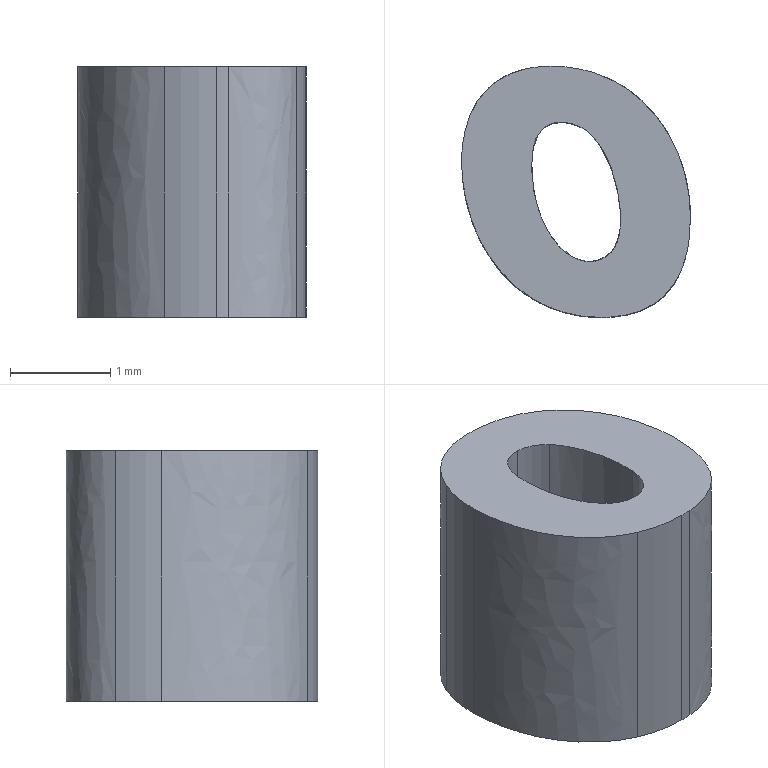Part | STEP file | lll_id1102_x_t | 1 solid | 17 faces | box 2.284 x 2.506 x 2.5 mm | volume 8.969 mm3 | other 9 | cylinder 6 | plane 2 | commonest cylinder face diameters 0.868 x1 2.315 x1 2.359 x1 2.639 x1 2.788 x1 2.85 x1
STEP:
#1=CARTESIAN_POINT('',(389.013,-124.465,2.35));
#2=VERTEX_POINT('',#1);
#3=CARTESIAN_POINT('',(389.328,-124.131,2.35));
#4=VERTEX_POINT('',#3);
#5=CARTESIAN_POINT('',(389.013,-124.465,2.35));
#6=CARTESIAN_POINT('',(389.141,-124.473,2.35));
#7=CARTESIAN_POINT('',(389.249,-124.404,2.35));
#8=CARTESIAN_POINT('',(389.303,-124.262,2.35));
#9=CARTESIAN_POINT('',(389.31,-124.24,2.35));
#10=CARTESIAN_POINT('',(389.322,-124.188,2.35));
#11=CARTESIAN_POINT('',(389.326,-124.16,2.35));
#12=CARTESIAN_POINT('',(389.328,-124.131,2.35));
#13=(BOUNDED_CURVE()B_SPLINE_CURVE(3,(#5,#6,#7,#8,#9,#10,#11,#12),.UNSPECIFIED.,.F.,.F.)B_SPLINE_CURVE_WITH_KNOTS((4,2,2,4),(0.,0.7103,0.842,1.),.UNSPECIFIED.)CURVE()GEOMETRIC_REPRESENTATION_ITEM()RATIONAL_B_SPLINE_CURVE((0.5541,0.482,0.482,0.5529,0.5529,0.5533,0.5533,0.5541))REPRESENTATION_ITEM(''));
#14=EDGE_CURVE('',#2,#4,#13,.T.);
#15=ORIENTED_EDGE('',*,*,#14,.T.);
#16=CARTESIAN_POINT('',(389.328,-124.131,-0.15));
#17=VERTEX_POINT('',#16);
#18=CARTESIAN_POINT('',(389.328,-124.131,-0.15));
#19=DIRECTION('',(0.,0.,1.));
#20=VECTOR('',#19,1.);
#21=LINE('',#18,#20);
#22=EDGE_CURVE('',#17,#4,#21,.T.);
#23=ORIENTED_EDGE('',*,*,#22,.F.);
#24=CARTESIAN_POINT('',(389.013,-124.465,-0.15));
#25=VERTEX_POINT('',#24);
#26=CARTESIAN_POINT('',(389.013,-124.465,-0.15));
#27=CARTESIAN_POINT('',(389.141,-124.473,-0.15));
#28=CARTESIAN_POINT('',(389.249,-124.404,-0.15));
#29=CARTESIAN_POINT('',(389.303,-124.262,-0.15));
#30=CARTESIAN_POINT('',(389.31,-124.24,-0.15));
#31=CARTESIAN_POINT('',(389.322,-124.188,-0.15));
#32=CARTESIAN_POINT('',(389.326,-124.16,-0.15));
#33=CARTESIAN_POINT('',(389.328,-124.131,-0.15));
#34=(BOUNDED_CURVE()B_SPLINE_CURVE(3,(#26,#27,#28,#29,#30,#31,#32,#33),.UNSPECIFIED.,.F.,.F.)B_SPLINE_CURVE_WITH_KNOTS((4,2,2,4),(0.,0.7103,0.842,1.),.UNSPECIFIED.)CURVE()GEOMETRIC_REPRESENTATION_ITEM()RATIONAL_B_SPLINE_CURVE((0.5541,0.482,0.482,0.5529,0.5529,0.5533,0.5533,0.5541))REPRESENTATION_ITEM(''));
#35=EDGE_CURVE('',#25,#17,#34,.T.);
#36=ORIENTED_EDGE('',*,*,#35,.F.);
#37=CARTESIAN_POINT('',(389.013,-124.465,-0.15));
#38=DIRECTION('',(0.,0.,1.));
#39=VECTOR('',#38,1.);
#40=LINE('',#37,#39);
#41=EDGE_CURVE('',#25,#2,#40,.T.);
#42=ORIENTED_EDGE('',*,*,#41,.T.);
#43=EDGE_LOOP('',(#15,#23,#36,#42));
#44=FACE_OUTER_BOUND('',#43,.T.);
#45=CARTESIAN_POINT('',(389.013,-124.465,-0.15));
#46=CARTESIAN_POINT('',(389.141,-124.473,-0.15));
#47=CARTESIAN_POINT('',(389.249,-124.404,-0.15));
#48=CARTESIAN_POINT('',(389.303,-124.262,-0.15));
#49=CARTESIAN_POINT('',(389.31,-124.24,-0.15));
#50=CARTESIAN_POINT('',(389.322,-124.188,-0.15));
#51=CARTESIAN_POINT('',(389.326,-124.16,-0.15));
#52=CARTESIAN_POINT('',(389.328,-124.131,-0.15));
#53=(BOUNDED_CURVE()B_SPLINE_CURVE(3,(#45,#46,#47,#48,#49,#50,#51,#52),.UNSPECIFIED.,.F.,.F.)B_SPLINE_CURVE_WITH_KNOTS((4,2,2,4),(0.,0.7103,0.842,1.),.UNSPECIFIED.)CURVE()GEOMETRIC_REPRESENTATION_ITEM()RATIONAL_B_SPLINE_CURVE((0.5541,0.482,0.482,0.5529,0.5529,0.5533,0.5533,0.5541))REPRESENTATION_ITEM(''));
#54=DIRECTION('',(0.,0.,1.));
#55=VECTOR('',#54,1.);
#56=SURFACE_OF_LINEAR_EXTRUSION('',#53,#55);
#57=ADVANCED_FACE('',(#44),#56,.F.);
#58=CARTESIAN_POINT('',(389.062,-123.223,2.35));
#59=VERTEX_POINT('',#58);
#60=CARTESIAN_POINT('',(389.328,-124.131,2.35));
#61=CARTESIAN_POINT('',(389.337,-124.008,2.35));
#62=CARTESIAN_POINT('',(389.329,-123.884,2.35));
#63=CARTESIAN_POINT('',(389.288,-123.679,2.35));
#64=CARTESIAN_POINT('',(389.265,-123.597,2.35));
#65=CARTESIAN_POINT('',(389.208,-123.446,2.35));
#66=CARTESIAN_POINT('',(389.173,-123.378,2.35));
#67=CARTESIAN_POINT('',(389.111,-123.282,2.35));
#68=CARTESIAN_POINT('',(389.088,-123.252,2.35));
#69=CARTESIAN_POINT('',(389.062,-123.223,2.35));
#70=(BOUNDED_CURVE()B_SPLINE_CURVE(3,(#60,#61,#62,#63,#64,#65,#66,#67,#68,#69),.UNSPECIFIED.,.F.,.F.)B_SPLINE_CURVE_WITH_KNOTS((4,2,2,2,4),(0.,0.3838,0.6481,0.8827,1.),.UNSPECIFIED.)CURVE()GEOMETRIC_REPRESENTATION_ITEM()RATIONAL_B_SPLINE_CURVE((0.5541,0.5507,0.5507,0.5528,0.5528,0.5521,0.5521,0.5529,0.5529,0.5541))REPRESENTATION_ITEM(''));
#71=EDGE_CURVE('',#4,#59,#70,.T.);
#72=ORIENTED_EDGE('',*,*,#71,.T.);
#73=CARTESIAN_POINT('',(389.062,-123.223,-0.15));
#74=VERTEX_POINT('',#73);
#75=CARTESIAN_POINT('',(389.062,-123.223,-0.15));
#76=DIRECTION('',(0.,0.,1.));
#77=VECTOR('',#76,1.);
#78=LINE('',#75,#77);
#79=EDGE_CURVE('',#74,#59,#78,.T.);
#80=ORIENTED_EDGE('',*,*,#79,.F.);
#81=CARTESIAN_POINT('',(389.328,-124.131,-0.15));
#82=CARTESIAN_POINT('',(389.337,-124.008,-0.15));
#83=CARTESIAN_POINT('',(389.329,-123.884,-0.15));
#84=CARTESIAN_POINT('',(389.288,-123.679,-0.15));
#85=CARTESIAN_POINT('',(389.265,-123.597,-0.15));
#86=CARTESIAN_POINT('',(389.208,-123.446,-0.15));
#87=CARTESIAN_POINT('',(389.173,-123.378,-0.15));
#88=CARTESIAN_POINT('',(389.111,-123.282,-0.15));
#89=CARTESIAN_POINT('',(389.088,-123.252,-0.15));
#90=CARTESIAN_POINT('',(389.062,-123.223,-0.15));
#91=(BOUNDED_CURVE()B_SPLINE_CURVE(3,(#81,#82,#83,#84,#85,#86,#87,#88,#89,#90),.UNSPECIFIED.,.F.,.F.)B_SPLINE_CURVE_WITH_KNOTS((4,2,2,2,4),(0.,0.3838,0.6481,0.8827,1.),.UNSPECIFIED.)CURVE()GEOMETRIC_REPRESENTATION_ITEM()RATIONAL_B_SPLINE_CURVE((0.5541,0.5507,0.5507,0.5528,0.5528,0.5521,0.5521,0.5529,0.5529,0.5541))REPRESENTATION_ITEM(''));
#92=EDGE_CURVE('',#17,#74,#91,.T.);
#93=ORIENTED_EDGE('',*,*,#92,.F.);
#94=ORIENTED_EDGE('',*,*,#22,.T.);
#95=EDGE_LOOP('',(#72,#80,#93,#94));
#96=FACE_OUTER_BOUND('',#95,.T.);
#97=CARTESIAN_POINT('',(389.328,-124.131,-0.15));
#98=CARTESIAN_POINT('',(389.337,-124.008,-0.15));
#99=CARTESIAN_POINT('',(389.329,-123.884,-0.15));
#100=CARTESIAN_POINT('',(389.288,-123.679,-0.15));
#101=CARTESIAN_POINT('',(389.265,-123.597,-0.15));
#102=CARTESIAN_POINT('',(389.208,-123.446,-0.15));
#103=CARTESIAN_POINT('',(389.173,-123.378,-0.15));
#104=CARTESIAN_POINT('',(389.111,-123.282,-0.15));
#105=CARTESIAN_POINT('',(389.088,-123.252,-0.15));
#106=CARTESIAN_POINT('',(389.062,-123.223,-0.15));
#107=(BOUNDED_CURVE()B_SPLINE_CURVE(3,(#97,#98,#99,#100,#101,#102,#103,#104,#105,#106),.UNSPECIFIED.,.F.,.F.)B_SPLINE_CURVE_WITH_KNOTS((4,2,2,2,4),(0.,0.3838,0.6481,0.8827,1.),.UNSPECIFIED.)CURVE()GEOMETRIC_REPRESENTATION_ITEM()RATIONAL_B_SPLINE_CURVE((0.5541,0.5507,0.5507,0.5528,0.5528,0.5521,0.5521,0.5529,0.5529,0.5541))REPRESENTATION_ITEM(''));
#108=DIRECTION('',(0.,0.,1.));
#109=VECTOR('',#108,1.);
#110=SURFACE_OF_LINEAR_EXTRUSION('',#107,#109);
#111=ADVANCED_FACE('',(#96),#110,.F.);
#112=CARTESIAN_POINT('',(388.763,-123.075,2.35));
#113=VERTEX_POINT('',#112);
#114=CARTESIAN_POINT('',(388.735,-123.509,2.35));
#115=DIRECTION('',(0.,0.,1.));
#116=DIRECTION('',(-1.,0.,0.));
#117=AXIS2_PLACEMENT_3D('',#114,#115,#116);
#118=CIRCLE('',#117,0.4341);
#119=EDGE_CURVE('',#59,#113,#118,.T.);
#120=ORIENTED_EDGE('',*,*,#119,.T.);
#121=CARTESIAN_POINT('',(388.763,-123.075,-0.15));
#122=VERTEX_POINT('',#121);
#123=CARTESIAN_POINT('',(388.763,-123.075,-0.15));
#124=DIRECTION('',(0.,0.,1.));
#125=VECTOR('',#124,1.);
#126=LINE('',#123,#125);
#127=EDGE_CURVE('',#122,#113,#126,.T.);
#128=ORIENTED_EDGE('',*,*,#127,.F.);
#129=CARTESIAN_POINT('',(388.735,-123.509,-0.15));
#130=DIRECTION('',(0.,0.,1.));
#131=DIRECTION('',(-1.,0.,0.));
#132=AXIS2_PLACEMENT_3D('',#129,#130,#131);
#133=CIRCLE('',#132,0.4341);
#134=EDGE_CURVE('',#74,#122,#133,.T.);
#135=ORIENTED_EDGE('',*,*,#134,.F.);
#136=ORIENTED_EDGE('',*,*,#79,.T.);
#137=EDGE_LOOP('',(#120,#128,#135,#136));
#138=FACE_OUTER_BOUND('',#137,.T.);
#139=CARTESIAN_POINT('',(388.735,-123.509,-0.15));
#140=DIRECTION('',(0.,0.,1.));
#141=DIRECTION('',(1.,0.,0.));
#142=AXIS2_PLACEMENT_3D('',#139,#140,#141);
#143=CYLINDRICAL_SURFACE('',#142,0.4341);
#144=ADVANCED_FACE('',(#138),#143,.F.);
#145=CARTESIAN_POINT('',(388.716,-124.311,2.35));
#146=VERTEX_POINT('',#145);
#147=CARTESIAN_POINT('',(388.763,-123.075,2.35));
#148=CARTESIAN_POINT('',(388.73,-123.073,2.35));
#149=CARTESIAN_POINT('',(388.696,-123.076,2.35));
#150=CARTESIAN_POINT('',(388.597,-123.1,2.35));
#151=CARTESIAN_POINT('',(388.542,-123.142,2.35));
#152=CARTESIAN_POINT('',(388.494,-123.227,2.35));
#153=CARTESIAN_POINT('',(388.483,-123.253,2.35));
#154=CARTESIAN_POINT('',(388.468,-123.304,2.35));
#155=CARTESIAN_POINT('',(388.463,-123.327,2.35));
#156=CARTESIAN_POINT('',(388.452,-123.388,2.35));
#157=CARTESIAN_POINT('',(388.448,-123.425,2.35));
#158=CARTESIAN_POINT('',(388.442,-123.606,2.35));
#159=CARTESIAN_POINT('',(388.459,-123.748,2.35));
#160=CARTESIAN_POINT('',(388.521,-123.987,2.35));
#161=CARTESIAN_POINT('',(388.562,-124.083,2.35));
#162=CARTESIAN_POINT('',(388.644,-124.222,2.35));
#163=CARTESIAN_POINT('',(388.678,-124.268,2.35));
#164=CARTESIAN_POINT('',(388.716,-124.311,2.35));
#165=(BOUNDED_CURVE()B_SPLINE_CURVE(3,(#147,#148,#149,#150,#151,#152,#153,#154,#155,#156,#157,#158,#159,#160,#161,#162,#163,#164),.UNSPECIFIED.,.F.,.F.)B_SPLINE_CURVE_WITH_KNOTS((4,2,2,2,2,2,2,2,4),(0.,0.07186,0.2116,0.2696,0.3174,0.394,0.6791,0.8867,1.),.UNSPECIFIED.)CURVE()GEOMETRIC_REPRESENTATION_ITEM()RATIONAL_B_SPLINE_CURVE((0.5028,0.4991,0.4991,0.4753,0.4753,0.5004,0.5004,0.5022,0.5022,0.502,0.502,0.4993,0.4993,0.4997,0.4997,0.5011,0.5011,0.5028))REPRESENTATION_ITEM(''));
#166=EDGE_CURVE('',#113,#146,#165,.T.);
#167=ORIENTED_EDGE('',*,*,#166,.T.);
#168=CARTESIAN_POINT('',(388.716,-124.311,-0.15));
#169=VERTEX_POINT('',#168);
#170=CARTESIAN_POINT('',(388.716,-124.311,-0.15));
#171=DIRECTION('',(0.,0.,1.));
#172=VECTOR('',#171,1.);
#173=LINE('',#170,#172);
#174=EDGE_CURVE('',#169,#146,#173,.T.);
#175=ORIENTED_EDGE('',*,*,#174,.F.);
#176=CARTESIAN_POINT('',(388.763,-123.075,-0.15));
#177=CARTESIAN_POINT('',(388.73,-123.073,-0.15));
#178=CARTESIAN_POINT('',(388.696,-123.076,-0.15));
#179=CARTESIAN_POINT('',(388.597,-123.1,-0.15));
#180=CARTESIAN_POINT('',(388.542,-123.142,-0.15));
#181=CARTESIAN_POINT('',(388.494,-123.227,-0.15));
#182=CARTESIAN_POINT('',(388.483,-123.253,-0.15));
#183=CARTESIAN_POINT('',(388.468,-123.304,-0.15));
#184=CARTESIAN_POINT('',(388.463,-123.327,-0.15));
#185=CARTESIAN_POINT('',(388.452,-123.388,-0.15));
#186=CARTESIAN_POINT('',(388.448,-123.425,-0.15));
#187=CARTESIAN_POINT('',(388.442,-123.606,-0.15));
#188=CARTESIAN_POINT('',(388.459,-123.748,-0.15));
#189=CARTESIAN_POINT('',(388.521,-123.987,-0.15));
#190=CARTESIAN_POINT('',(388.562,-124.083,-0.15));
#191=CARTESIAN_POINT('',(388.644,-124.222,-0.15));
#192=CARTESIAN_POINT('',(388.678,-124.268,-0.15));
#193=CARTESIAN_POINT('',(388.716,-124.311,-0.15));
#194=(BOUNDED_CURVE()B_SPLINE_CURVE(3,(#176,#177,#178,#179,#180,#181,#182,#183,#184,#185,#186,#187,#188,#189,#190,#191,#192,#193),.UNSPECIFIED.,.F.,.F.)B_SPLINE_CURVE_WITH_KNOTS((4,2,2,2,2,2,2,2,4),(0.,0.07186,0.2116,0.2696,0.3174,0.394,0.6791,0.8867,1.),.UNSPECIFIED.)CURVE()GEOMETRIC_REPRESENTATION_ITEM()RATIONAL_B_SPLINE_CURVE((0.5028,0.4991,0.4991,0.4753,0.4753,0.5004,0.5004,0.5022,0.5022,0.502,0.502,0.4993,0.4993,0.4997,0.4997,0.5011,0.5011,0.5028))REPRESENTATION_ITEM(''));
#195=EDGE_CURVE('',#122,#169,#194,.T.);
#196=ORIENTED_EDGE('',*,*,#195,.F.);
#197=ORIENTED_EDGE('',*,*,#127,.T.);
#198=EDGE_LOOP('',(#167,#175,#196,#197));
#199=FACE_OUTER_BOUND('',#198,.T.);
#200=CARTESIAN_POINT('',(388.763,-123.075,-0.15));
#201=CARTESIAN_POINT('',(388.73,-123.073,-0.15));
#202=CARTESIAN_POINT('',(388.696,-123.076,-0.15));
#203=CARTESIAN_POINT('',(388.597,-123.1,-0.15));
#204=CARTESIAN_POINT('',(388.542,-123.142,-0.15));
#205=CARTESIAN_POINT('',(388.494,-123.227,-0.15));
#206=CARTESIAN_POINT('',(388.483,-123.253,-0.15));
#207=CARTESIAN_POINT('',(388.468,-123.304,-0.15));
#208=CARTESIAN_POINT('',(388.463,-123.327,-0.15));
#209=CARTESIAN_POINT('',(388.452,-123.388,-0.15));
#210=CARTESIAN_POINT('',(388.448,-123.425,-0.15));
#211=CARTESIAN_POINT('',(388.442,-123.606,-0.15));
#212=CARTESIAN_POINT('',(388.459,-123.748,-0.15));
#213=CARTESIAN_POINT('',(388.521,-123.987,-0.15));
#214=CARTESIAN_POINT('',(388.562,-124.083,-0.15));
#215=CARTESIAN_POINT('',(388.644,-124.222,-0.15));
#216=CARTESIAN_POINT('',(388.678,-124.268,-0.15));
#217=CARTESIAN_POINT('',(388.716,-124.311,-0.15));
#218=(BOUNDED_CURVE()B_SPLINE_CURVE(3,(#200,#201,#202,#203,#204,#205,#206,#207,#208,#209,#210,#211,#212,#213,#214,#215,#216,#217),.UNSPECIFIED.,.F.,.F.)B_SPLINE_CURVE_WITH_KNOTS((4,2,2,2,2,2,2,2,4),(0.,0.07186,0.2116,0.2696,0.3174,0.394,0.6791,0.8867,1.),.UNSPECIFIED.)CURVE()GEOMETRIC_REPRESENTATION_ITEM()RATIONAL_B_SPLINE_CURVE((0.5028,0.4991,0.4991,0.4753,0.4753,0.5004,0.5004,0.5022,0.5022,0.502,0.502,0.4993,0.4993,0.4997,0.4997,0.5011,0.5011,0.5028))REPRESENTATION_ITEM(''));
#219=DIRECTION('',(0.,0.,1.));
#220=VECTOR('',#219,1.);
#221=SURFACE_OF_LINEAR_EXTRUSION('',#218,#220);
#222=ADVANCED_FACE('',(#199),#221,.F.);
#223=CARTESIAN_POINT('',(388.984,-124.463,2.35));
#224=VERTEX_POINT('',#223);
#225=CARTESIAN_POINT('',(388.716,-124.311,2.35));
#226=CARTESIAN_POINT('',(388.757,-124.358,2.35));
#227=CARTESIAN_POINT('',(388.806,-124.396,2.35));
#228=CARTESIAN_POINT('',(388.9,-124.446,2.35));
#229=CARTESIAN_POINT('',(388.941,-124.459,2.35));
#230=CARTESIAN_POINT('',(388.984,-124.463,2.35));
#231=(BOUNDED_CURVE()B_SPLINE_CURVE(3,(#225,#226,#227,#228,#229,#230),.UNSPECIFIED.,.F.,.F.)B_SPLINE_CURVE_WITH_KNOTS((4,2,4),(0.,0.5929,1.),.UNSPECIFIED.)CURVE()GEOMETRIC_REPRESENTATION_ITEM()RATIONAL_B_SPLINE_CURVE((0.5028,0.4974,0.4974,0.497,0.497,0.5028))REPRESENTATION_ITEM(''));
#232=EDGE_CURVE('',#146,#224,#231,.T.);
#233=ORIENTED_EDGE('',*,*,#232,.T.);
#234=CARTESIAN_POINT('',(388.984,-124.463,-0.15));
#235=VERTEX_POINT('',#234);
#236=CARTESIAN_POINT('',(388.984,-124.463,-0.15));
#237=DIRECTION('',(0.,0.,1.));
#238=VECTOR('',#237,1.);
#239=LINE('',#236,#238);
#240=EDGE_CURVE('',#235,#224,#239,.T.);
#241=ORIENTED_EDGE('',*,*,#240,.F.);
#242=CARTESIAN_POINT('',(388.716,-124.311,-0.15));
#243=CARTESIAN_POINT('',(388.757,-124.358,-0.15));
#244=CARTESIAN_POINT('',(388.806,-124.396,-0.15));
#245=CARTESIAN_POINT('',(388.9,-124.446,-0.15));
#246=CARTESIAN_POINT('',(388.941,-124.459,-0.15));
#247=CARTESIAN_POINT('',(388.984,-124.463,-0.15));
#248=(BOUNDED_CURVE()B_SPLINE_CURVE(3,(#242,#243,#244,#245,#246,#247),.UNSPECIFIED.,.F.,.F.)B_SPLINE_CURVE_WITH_KNOTS((4,2,4),(0.,0.5929,1.),.UNSPECIFIED.)CURVE()GEOMETRIC_REPRESENTATION_ITEM()RATIONAL_B_SPLINE_CURVE((0.5028,0.4974,0.4974,0.497,0.497,0.5028))REPRESENTATION_ITEM(''));
#249=EDGE_CURVE('',#169,#235,#248,.T.);
#250=ORIENTED_EDGE('',*,*,#249,.F.);
#251=ORIENTED_EDGE('',*,*,#174,.T.);
#252=EDGE_LOOP('',(#233,#241,#250,#251));
#253=FACE_OUTER_BOUND('',#252,.T.);
#254=CARTESIAN_POINT('',(388.716,-124.311,-0.15));
#255=CARTESIAN_POINT('',(388.757,-124.358,-0.15));
#256=CARTESIAN_POINT('',(388.806,-124.396,-0.15));
#257=CARTESIAN_POINT('',(388.9,-124.446,-0.15));
#258=CARTESIAN_POINT('',(388.941,-124.459,-0.15));
#259=CARTESIAN_POINT('',(388.984,-124.463,-0.15));
#260=(BOUNDED_CURVE()B_SPLINE_CURVE(3,(#254,#255,#256,#257,#258,#259),.UNSPECIFIED.,.F.,.F.)B_SPLINE_CURVE_WITH_KNOTS((4,2,4),(0.,0.5929,1.),.UNSPECIFIED.)CURVE()GEOMETRIC_REPRESENTATION_ITEM()RATIONAL_B_SPLINE_CURVE((0.5028,0.4974,0.4974,0.497,0.497,0.5028))REPRESENTATION_ITEM(''));
#261=DIRECTION('',(0.,0.,1.));
#262=VECTOR('',#261,1.);
#263=SURFACE_OF_LINEAR_EXTRUSION('',#260,#262);
#264=ADVANCED_FACE('',(#253),#263,.F.);
#265=CARTESIAN_POINT('',(388.65,-122.517,2.35));
#266=VERTEX_POINT('',#265);
#267=CARTESIAN_POINT('',(389.061,-122.579,2.35));
#268=VERTEX_POINT('',#267);
#269=CARTESIAN_POINT('',(388.645,-123.942,2.35));
#270=DIRECTION('',(0.,0.,-1.));
#271=DIRECTION('',(0.,-1.,0.));
#272=AXIS2_PLACEMENT_3D('',#269,#270,#271);
#273=CIRCLE('',#272,1.425);
#274=EDGE_CURVE('',#266,#268,#273,.T.);
#275=ORIENTED_EDGE('',*,*,#274,.T.);
#276=CARTESIAN_POINT('',(389.061,-122.579,-0.15));
#277=VERTEX_POINT('',#276);
#278=CARTESIAN_POINT('',(389.061,-122.579,-0.15));
#279=DIRECTION('',(0.,0.,1.));
#280=VECTOR('',#279,1.);
#281=LINE('',#278,#280);
#282=EDGE_CURVE('',#277,#268,#281,.T.);
#283=ORIENTED_EDGE('',*,*,#282,.F.);
#284=CARTESIAN_POINT('',(388.65,-122.517,-0.15));
#285=VERTEX_POINT('',#284);
#286=CARTESIAN_POINT('',(388.645,-123.942,-0.15));
#287=DIRECTION('',(0.,0.,-1.));
#288=DIRECTION('',(1.,0.,0.));
#289=AXIS2_PLACEMENT_3D('',#286,#287,#288);
#290=CIRCLE('',#289,1.425);
#291=EDGE_CURVE('',#285,#277,#290,.T.);
#292=ORIENTED_EDGE('',*,*,#291,.F.);
#293=CARTESIAN_POINT('',(388.65,-122.517,-0.15));
#294=DIRECTION('',(0.,0.,1.));
#295=VECTOR('',#294,1.);
#296=LINE('',#293,#295);
#297=EDGE_CURVE('',#285,#266,#296,.T.);
#298=ORIENTED_EDGE('',*,*,#297,.T.);
#299=EDGE_LOOP('',(#275,#283,#292,#298));
#300=FACE_OUTER_BOUND('',#299,.T.);
#301=CARTESIAN_POINT('',(388.645,-123.942,-0.15));
#302=DIRECTION('',(0.,0.,1.));
#303=DIRECTION('',(1.,0.,0.));
#304=AXIS2_PLACEMENT_3D('',#301,#302,#303);
#305=CYLINDRICAL_SURFACE('',#304,1.425);
#306=ADVANCED_FACE('',(#300),#305,.T.);
#307=CARTESIAN_POINT('',(390.017,-124.245,2.35));
#308=VERTEX_POINT('',#307);
#309=CARTESIAN_POINT('',(389.061,-122.579,2.35));
#310=CARTESIAN_POINT('',(389.291,-122.652,2.35));
#311=CARTESIAN_POINT('',(389.492,-122.785,2.35));
#312=CARTESIAN_POINT('',(389.805,-123.151,2.35));
#313=CARTESIAN_POINT('',(389.917,-123.363,2.35));
#314=CARTESIAN_POINT('',(390.03,-123.808,2.35));
#315=CARTESIAN_POINT('',(390.044,-124.028,2.35));
#316=CARTESIAN_POINT('',(390.017,-124.245,2.35));
#317=(BOUNDED_CURVE()B_SPLINE_CURVE(3,(#309,#310,#311,#312,#313,#314,#315,#316),.UNSPECIFIED.,.F.,.F.)B_SPLINE_CURVE_WITH_KNOTS((4,2,2,4),(0.,0.3492,0.691,1.),.UNSPECIFIED.)CURVE()GEOMETRIC_REPRESENTATION_ITEM()RATIONAL_B_SPLINE_CURVE((0.5027,0.4899,0.4899,0.4938,0.4938,0.4968,0.4968,0.5027))REPRESENTATION_ITEM(''));
#318=EDGE_CURVE('',#268,#308,#317,.T.);
#319=ORIENTED_EDGE('',*,*,#318,.T.);
#320=CARTESIAN_POINT('',(390.017,-124.245,-0.15));
#321=VERTEX_POINT('',#320);
#322=CARTESIAN_POINT('',(390.017,-124.245,-0.15));
#323=DIRECTION('',(0.,0.,1.));
#324=VECTOR('',#323,1.);
#325=LINE('',#322,#324);
#326=EDGE_CURVE('',#321,#308,#325,.T.);
#327=ORIENTED_EDGE('',*,*,#326,.F.);
#328=CARTESIAN_POINT('',(389.061,-122.579,-0.15));
#329=CARTESIAN_POINT('',(389.291,-122.652,-0.15));
#330=CARTESIAN_POINT('',(389.492,-122.785,-0.15));
#331=CARTESIAN_POINT('',(389.805,-123.151,-0.15));
#332=CARTESIAN_POINT('',(389.917,-123.363,-0.15));
#333=CARTESIAN_POINT('',(390.03,-123.808,-0.15));
#334=CARTESIAN_POINT('',(390.044,-124.028,-0.15));
#335=CARTESIAN_POINT('',(390.017,-124.245,-0.15));
#336=(BOUNDED_CURVE()B_SPLINE_CURVE(3,(#328,#329,#330,#331,#332,#333,#334,#335),.UNSPECIFIED.,.F.,.F.)B_SPLINE_CURVE_WITH_KNOTS((4,2,2,4),(0.,0.3492,0.691,1.),.UNSPECIFIED.)CURVE()GEOMETRIC_REPRESENTATION_ITEM()RATIONAL_B_SPLINE_CURVE((0.5027,0.4899,0.4899,0.4938,0.4938,0.4968,0.4968,0.5027))REPRESENTATION_ITEM(''));
#337=EDGE_CURVE('',#277,#321,#336,.T.);
#338=ORIENTED_EDGE('',*,*,#337,.F.);
#339=ORIENTED_EDGE('',*,*,#282,.T.);
#340=EDGE_LOOP('',(#319,#327,#338,#339));
#341=FACE_OUTER_BOUND('',#340,.T.);
#342=CARTESIAN_POINT('',(389.061,-122.579,-0.15));
#343=CARTESIAN_POINT('',(389.291,-122.652,-0.15));
#344=CARTESIAN_POINT('',(389.492,-122.785,-0.15));
#345=CARTESIAN_POINT('',(389.805,-123.151,-0.15));
#346=CARTESIAN_POINT('',(389.917,-123.363,-0.15));
#347=CARTESIAN_POINT('',(390.03,-123.808,-0.15));
#348=CARTESIAN_POINT('',(390.044,-124.028,-0.15));
#349=CARTESIAN_POINT('',(390.017,-124.245,-0.15));
#350=(BOUNDED_CURVE()B_SPLINE_CURVE(3,(#342,#343,#344,#345,#346,#347,#348,#349),.UNSPECIFIED.,.F.,.F.)B_SPLINE_CURVE_WITH_KNOTS((4,2,2,4),(0.,0.3492,0.691,1.),.UNSPECIFIED.)CURVE()GEOMETRIC_REPRESENTATION_ITEM()RATIONAL_B_SPLINE_CURVE((0.5027,0.4899,0.4899,0.4938,0.4938,0.4968,0.4968,0.5027))REPRESENTATION_ITEM(''));
#351=DIRECTION('',(0.,0.,1.));
#352=VECTOR('',#351,1.);
#353=SURFACE_OF_LINEAR_EXTRUSION('',#350,#352);
#354=ADVANCED_FACE('',(#341),#353,.F.);
#355=CARTESIAN_POINT('',(389.934,-124.562,2.35));
#356=VERTEX_POINT('',#355);
#357=CARTESIAN_POINT('',(388.845,-124.109,2.35));
#358=DIRECTION('',(0.,0.,-1.));
#359=DIRECTION('',(1.,0.,0.));
#360=AXIS2_PLACEMENT_3D('',#357,#358,#359);
#361=CIRCLE('',#360,1.179);
#362=EDGE_CURVE('',#308,#356,#361,.T.);
#363=ORIENTED_EDGE('',*,*,#362,.T.);
#364=CARTESIAN_POINT('',(389.934,-124.562,-0.15));
#365=VERTEX_POINT('',#364);
#366=CARTESIAN_POINT('',(389.934,-124.562,-0.15));
#367=DIRECTION('',(0.,0.,1.));
#368=VECTOR('',#367,1.);
#369=LINE('',#366,#368);
#370=EDGE_CURVE('',#365,#356,#369,.T.);
#371=ORIENTED_EDGE('',*,*,#370,.F.);
#372=CARTESIAN_POINT('',(388.845,-124.109,-0.15));
#373=DIRECTION('',(0.,0.,-1.));
#374=DIRECTION('',(1.,0.,0.));
#375=AXIS2_PLACEMENT_3D('',#372,#373,#374);
#376=CIRCLE('',#375,1.179);
#377=EDGE_CURVE('',#321,#365,#376,.T.);
#378=ORIENTED_EDGE('',*,*,#377,.F.);
#379=ORIENTED_EDGE('',*,*,#326,.T.);
#380=EDGE_LOOP('',(#363,#371,#378,#379));
#381=FACE_OUTER_BOUND('',#380,.T.);
#382=CARTESIAN_POINT('',(388.845,-124.109,-0.15));
#383=DIRECTION('',(0.,0.,1.));
#384=DIRECTION('',(1.,0.,0.));
#385=AXIS2_PLACEMENT_3D('',#382,#383,#384);
#386=CYLINDRICAL_SURFACE('',#385,1.179);
#387=ADVANCED_FACE('',(#381),#386,.T.);
#388=CARTESIAN_POINT('',(389.253,-125.018,2.35));
#389=VERTEX_POINT('',#388);
#390=CARTESIAN_POINT('',(389.934,-124.562,2.35));
#391=CARTESIAN_POINT('',(389.857,-124.753,2.35));
#392=CARTESIAN_POINT('',(389.709,-124.895,2.35));
#393=CARTESIAN_POINT('',(389.43,-124.993,2.35));
#394=CARTESIAN_POINT('',(389.343,-125.011,2.35));
#395=CARTESIAN_POINT('',(389.253,-125.018,2.35));
#396=(BOUNDED_CURVE()B_SPLINE_CURVE(3,(#390,#391,#392,#393,#394,#395),.UNSPECIFIED.,.F.,.F.)B_SPLINE_CURVE_WITH_KNOTS((4,2,4),(0.,0.698,1.),.UNSPECIFIED.)CURVE()GEOMETRIC_REPRESENTATION_ITEM()RATIONAL_B_SPLINE_CURVE((0.5027,0.4728,0.4728,0.4997,0.4997,0.5027))REPRESENTATION_ITEM(''));
#397=EDGE_CURVE('',#356,#389,#396,.T.);
#398=ORIENTED_EDGE('',*,*,#397,.T.);
#399=CARTESIAN_POINT('',(389.253,-125.018,-0.15));
#400=VERTEX_POINT('',#399);
#401=CARTESIAN_POINT('',(389.253,-125.018,-0.15));
#402=DIRECTION('',(0.,0.,1.));
#403=VECTOR('',#402,1.);
#404=LINE('',#401,#403);
#405=EDGE_CURVE('',#400,#389,#404,.T.);
#406=ORIENTED_EDGE('',*,*,#405,.F.);
#407=CARTESIAN_POINT('',(389.934,-124.562,-0.15));
#408=CARTESIAN_POINT('',(389.857,-124.753,-0.15));
#409=CARTESIAN_POINT('',(389.709,-124.895,-0.15));
#410=CARTESIAN_POINT('',(389.43,-124.993,-0.15));
#411=CARTESIAN_POINT('',(389.343,-125.011,-0.15));
#412=CARTESIAN_POINT('',(389.253,-125.018,-0.15));
#413=(BOUNDED_CURVE()B_SPLINE_CURVE(3,(#407,#408,#409,#410,#411,#412),.UNSPECIFIED.,.F.,.F.)B_SPLINE_CURVE_WITH_KNOTS((4,2,4),(0.,0.698,1.),.UNSPECIFIED.)CURVE()GEOMETRIC_REPRESENTATION_ITEM()RATIONAL_B_SPLINE_CURVE((0.5027,0.4728,0.4728,0.4997,0.4997,0.5027))REPRESENTATION_ITEM(''));
#414=EDGE_CURVE('',#365,#400,#413,.T.);
#415=ORIENTED_EDGE('',*,*,#414,.F.);
#416=ORIENTED_EDGE('',*,*,#370,.T.);
#417=EDGE_LOOP('',(#398,#406,#415,#416));
#418=FACE_OUTER_BOUND('',#417,.T.);
#419=CARTESIAN_POINT('',(389.934,-124.562,-0.15));
#420=CARTESIAN_POINT('',(389.857,-124.753,-0.15));
#421=CARTESIAN_POINT('',(389.709,-124.895,-0.15));
#422=CARTESIAN_POINT('',(389.43,-124.993,-0.15));
#423=CARTESIAN_POINT('',(389.343,-125.011,-0.15));
#424=CARTESIAN_POINT('',(389.253,-125.018,-0.15));
#425=(BOUNDED_CURVE()B_SPLINE_CURVE(3,(#419,#420,#421,#422,#423,#424),.UNSPECIFIED.,.F.,.F.)B_SPLINE_CURVE_WITH_KNOTS((4,2,4),(0.,0.698,1.),.UNSPECIFIED.)CURVE()GEOMETRIC_REPRESENTATION_ITEM()RATIONAL_B_SPLINE_CURVE((0.5027,0.4728,0.4728,0.4997,0.4997,0.5027))REPRESENTATION_ITEM(''));
#426=DIRECTION('',(0.,0.,1.));
#427=VECTOR('',#426,1.);
#428=SURFACE_OF_LINEAR_EXTRUSION('',#425,#427);
#429=ADVANCED_FACE('',(#418),#428,.F.);
#430=CARTESIAN_POINT('',(389.135,-125.023,2.35));
#431=VERTEX_POINT('',#430);
#432=CARTESIAN_POINT('',(389.139,-123.629,2.35));
#433=DIRECTION('',(0.,0.,-1.));
#434=DIRECTION('',(0.,-1.,0.));
#435=AXIS2_PLACEMENT_3D('',#432,#433,#434);
#436=CIRCLE('',#435,1.394);
#437=EDGE_CURVE('',#389,#431,#436,.T.);
#438=ORIENTED_EDGE('',*,*,#437,.T.);
#439=CARTESIAN_POINT('',(389.135,-125.023,-0.15));
#440=VERTEX_POINT('',#439);
#441=CARTESIAN_POINT('',(389.135,-125.023,-0.15));
#442=DIRECTION('',(0.,0.,1.));
#443=VECTOR('',#442,1.);
#444=LINE('',#441,#443);
#445=EDGE_CURVE('',#440,#431,#444,.T.);
#446=ORIENTED_EDGE('',*,*,#445,.F.);
#447=CARTESIAN_POINT('',(389.139,-123.629,-0.15));
#448=DIRECTION('',(0.,0.,-1.));
#449=DIRECTION('',(0.,-1.,0.));
#450=AXIS2_PLACEMENT_3D('',#447,#448,#449);
#451=CIRCLE('',#450,1.394);
#452=EDGE_CURVE('',#400,#440,#451,.T.);
#453=ORIENTED_EDGE('',*,*,#452,.F.);
#454=ORIENTED_EDGE('',*,*,#405,.T.);
#455=EDGE_LOOP('',(#438,#446,#453,#454));
#456=FACE_OUTER_BOUND('',#455,.T.);
#457=CARTESIAN_POINT('',(389.139,-123.629,-0.15));
#458=DIRECTION('',(0.,0.,1.));
#459=DIRECTION('',(1.,0.,0.));
#460=AXIS2_PLACEMENT_3D('',#457,#458,#459);
#461=CYLINDRICAL_SURFACE('',#460,1.394);
#462=ADVANCED_FACE('',(#456),#461,.T.);
#463=CARTESIAN_POINT('',(388.612,-124.918,2.35));
#464=VERTEX_POINT('',#463);
#465=CARTESIAN_POINT('',(389.127,-123.703,2.35));
#466=DIRECTION('',(0.,0.,-1.));
#467=DIRECTION('',(1.,0.,0.));
#468=AXIS2_PLACEMENT_3D('',#465,#466,#467);
#469=CIRCLE('',#468,1.319);
#470=EDGE_CURVE('',#431,#464,#469,.T.);
#471=ORIENTED_EDGE('',*,*,#470,.T.);
#472=CARTESIAN_POINT('',(388.612,-124.918,-0.15));
#473=VERTEX_POINT('',#472);
#474=CARTESIAN_POINT('',(388.612,-124.918,-0.15));
#475=DIRECTION('',(0.,0.,1.));
#476=VECTOR('',#475,1.);
#477=LINE('',#474,#476);
#478=EDGE_CURVE('',#473,#464,#477,.T.);
#479=ORIENTED_EDGE('',*,*,#478,.F.);
#480=CARTESIAN_POINT('',(389.127,-123.703,-0.15));
#481=DIRECTION('',(0.,0.,-1.));
#482=DIRECTION('',(1.,0.,0.));
#483=AXIS2_PLACEMENT_3D('',#480,#481,#482);
#484=CIRCLE('',#483,1.319);
#485=EDGE_CURVE('',#440,#473,#484,.T.);
#486=ORIENTED_EDGE('',*,*,#485,.F.);
#487=ORIENTED_EDGE('',*,*,#445,.T.);
#488=EDGE_LOOP('',(#471,#479,#486,#487));
#489=FACE_OUTER_BOUND('',#488,.T.);
#490=CARTESIAN_POINT('',(389.127,-123.703,-0.15));
#491=DIRECTION('',(0.,0.,1.));
#492=DIRECTION('',(1.,0.,0.));
#493=AXIS2_PLACEMENT_3D('',#490,#491,#492);
#494=CYLINDRICAL_SURFACE('',#493,1.319);
#495=ADVANCED_FACE('',(#489),#494,.T.);
#496=CARTESIAN_POINT('',(387.746,-123.469,2.35));
#497=VERTEX_POINT('',#496);
#498=CARTESIAN_POINT('',(388.612,-124.918,2.35));
#499=CARTESIAN_POINT('',(388.41,-124.83,2.35));
#500=CARTESIAN_POINT('',(388.236,-124.695,2.35));
#501=CARTESIAN_POINT('',(387.99,-124.38,2.35));
#502=CARTESIAN_POINT('',(387.905,-124.222,2.35));
#503=CARTESIAN_POINT('',(387.783,-123.864,2.35));
#504=CARTESIAN_POINT('',(387.749,-123.668,2.35));
#505=CARTESIAN_POINT('',(387.746,-123.469,2.35));
#506=(BOUNDED_CURVE()B_SPLINE_CURVE(3,(#498,#499,#500,#501,#502,#503,#504,#505),.UNSPECIFIED.,.F.,.F.)B_SPLINE_CURVE_WITH_KNOTS((4,2,2,4),(0.,0.3712,0.6704,1.),.UNSPECIFIED.)CURVE()GEOMETRIC_REPRESENTATION_ITEM()RATIONAL_B_SPLINE_CURVE((0.5052,0.4949,0.4949,0.5005,0.5005,0.5009,0.5009,0.5052))REPRESENTATION_ITEM(''));
#507=EDGE_CURVE('',#464,#497,#506,.T.);
#508=ORIENTED_EDGE('',*,*,#507,.T.);
#509=CARTESIAN_POINT('',(387.746,-123.469,-0.15));
#510=VERTEX_POINT('',#509);
#511=CARTESIAN_POINT('',(387.746,-123.469,-0.15));
#512=DIRECTION('',(0.,0.,1.));
#513=VECTOR('',#512,1.);
#514=LINE('',#511,#513);
#515=EDGE_CURVE('',#510,#497,#514,.T.);
#516=ORIENTED_EDGE('',*,*,#515,.F.);
#517=CARTESIAN_POINT('',(388.612,-124.918,-0.15));
#518=CARTESIAN_POINT('',(388.41,-124.83,-0.15));
#519=CARTESIAN_POINT('',(388.236,-124.695,-0.15));
#520=CARTESIAN_POINT('',(387.99,-124.38,-0.15));
#521=CARTESIAN_POINT('',(387.905,-124.222,-0.15));
#522=CARTESIAN_POINT('',(387.783,-123.864,-0.15));
#523=CARTESIAN_POINT('',(387.749,-123.668,-0.15));
#524=CARTESIAN_POINT('',(387.746,-123.469,-0.15));
#525=(BOUNDED_CURVE()B_SPLINE_CURVE(3,(#517,#518,#519,#520,#521,#522,#523,#524),.UNSPECIFIED.,.F.,.F.)B_SPLINE_CURVE_WITH_KNOTS((4,2,2,4),(0.,0.3712,0.6704,1.),.UNSPECIFIED.)CURVE()GEOMETRIC_REPRESENTATION_ITEM()RATIONAL_B_SPLINE_CURVE((0.5052,0.4949,0.4949,0.5005,0.5005,0.5009,0.5009,0.5052))REPRESENTATION_ITEM(''));
#526=EDGE_CURVE('',#473,#510,#525,.T.);
#527=ORIENTED_EDGE('',*,*,#526,.F.);
#528=ORIENTED_EDGE('',*,*,#478,.T.);
#529=EDGE_LOOP('',(#508,#516,#527,#528));
#530=FACE_OUTER_BOUND('',#529,.T.);
#531=CARTESIAN_POINT('',(388.612,-124.918,-0.15));
#532=CARTESIAN_POINT('',(388.41,-124.83,-0.15));
#533=CARTESIAN_POINT('',(388.236,-124.695,-0.15));
#534=CARTESIAN_POINT('',(387.99,-124.38,-0.15));
#535=CARTESIAN_POINT('',(387.905,-124.222,-0.15));
#536=CARTESIAN_POINT('',(387.783,-123.864,-0.15));
#537=CARTESIAN_POINT('',(387.749,-123.668,-0.15));
#538=CARTESIAN_POINT('',(387.746,-123.469,-0.15));
#539=(BOUNDED_CURVE()B_SPLINE_CURVE(3,(#531,#532,#533,#534,#535,#536,#537,#538),.UNSPECIFIED.,.F.,.F.)B_SPLINE_CURVE_WITH_KNOTS((4,2,2,4),(0.,0.3712,0.6704,1.),.UNSPECIFIED.)CURVE()GEOMETRIC_REPRESENTATION_ITEM()RATIONAL_B_SPLINE_CURVE((0.5052,0.4949,0.4949,0.5005,0.5005,0.5009,0.5009,0.5052))REPRESENTATION_ITEM(''));
#540=DIRECTION('',(0.,0.,1.));
#541=VECTOR('',#540,1.);
#542=SURFACE_OF_LINEAR_EXTRUSION('',#539,#541);
#543=ADVANCED_FACE('',(#530),#542,.F.);
#544=CARTESIAN_POINT('',(387.833,-123.003,2.35));
#545=VERTEX_POINT('',#544);
#546=CARTESIAN_POINT('',(388.904,-123.444,2.35));
#547=DIRECTION('',(0.,0.,-1.));
#548=DIRECTION('',(1.,0.,0.));
#549=AXIS2_PLACEMENT_3D('',#546,#547,#548);
#550=CIRCLE('',#549,1.157);
#551=EDGE_CURVE('',#497,#545,#550,.T.);
#552=ORIENTED_EDGE('',*,*,#551,.T.);
#553=CARTESIAN_POINT('',(387.833,-123.003,-0.15));
#554=VERTEX_POINT('',#553);
#555=CARTESIAN_POINT('',(387.833,-123.003,-0.15));
#556=DIRECTION('',(0.,0.,1.));
#557=VECTOR('',#556,1.);
#558=LINE('',#555,#557);
#559=EDGE_CURVE('',#554,#545,#558,.T.);
#560=ORIENTED_EDGE('',*,*,#559,.F.);
#561=CARTESIAN_POINT('',(388.904,-123.444,-0.15));
#562=DIRECTION('',(0.,0.,-1.));
#563=DIRECTION('',(1.,0.,0.));
#564=AXIS2_PLACEMENT_3D('',#561,#562,#563);
#565=CIRCLE('',#564,1.157);
#566=EDGE_CURVE('',#510,#554,#565,.T.);
#567=ORIENTED_EDGE('',*,*,#566,.F.);
#568=ORIENTED_EDGE('',*,*,#515,.T.);
#569=EDGE_LOOP('',(#552,#560,#567,#568));
#570=FACE_OUTER_BOUND('',#569,.T.);
#571=CARTESIAN_POINT('',(388.904,-123.444,-0.15));
#572=DIRECTION('',(0.,0.,1.));
#573=DIRECTION('',(1.,0.,0.));
#574=AXIS2_PLACEMENT_3D('',#571,#572,#573);
#575=CYLINDRICAL_SURFACE('',#574,1.157);
#576=ADVANCED_FACE('',(#570),#575,.T.);
#577=CARTESIAN_POINT('',(387.833,-123.003,2.35));
#578=CARTESIAN_POINT('',(387.921,-122.783,2.35));
#579=CARTESIAN_POINT('',(388.098,-122.624,2.35));
#580=CARTESIAN_POINT('',(388.393,-122.54,2.35));
#581=CARTESIAN_POINT('',(388.462,-122.527,2.35));
#582=CARTESIAN_POINT('',(388.571,-122.518,2.35));
#583=CARTESIAN_POINT('',(388.61,-122.517,2.35));
#584=CARTESIAN_POINT('',(388.65,-122.517,2.35));
#585=(BOUNDED_CURVE()B_SPLINE_CURVE(3,(#577,#578,#579,#580,#581,#582,#583,#584),.UNSPECIFIED.,.F.,.F.)B_SPLINE_CURVE_WITH_KNOTS((4,2,2,4),(0.,0.6854,0.8859,1.),.UNSPECIFIED.)CURVE()GEOMETRIC_REPRESENTATION_ITEM()RATIONAL_B_SPLINE_CURVE((0.5052,0.4708,0.4708,0.5034,0.5034,0.5049,0.5049,0.5052))REPRESENTATION_ITEM(''));
#586=EDGE_CURVE('',#545,#266,#585,.T.);
#587=ORIENTED_EDGE('',*,*,#586,.T.);
#588=ORIENTED_EDGE('',*,*,#297,.F.);
#589=CARTESIAN_POINT('',(387.833,-123.003,-0.15));
#590=CARTESIAN_POINT('',(387.921,-122.783,-0.15));
#591=CARTESIAN_POINT('',(388.098,-122.624,-0.15));
#592=CARTESIAN_POINT('',(388.393,-122.54,-0.15));
#593=CARTESIAN_POINT('',(388.462,-122.527,-0.15));
#594=CARTESIAN_POINT('',(388.571,-122.518,-0.15));
#595=CARTESIAN_POINT('',(388.61,-122.517,-0.15));
#596=CARTESIAN_POINT('',(388.65,-122.517,-0.15));
#597=(BOUNDED_CURVE()B_SPLINE_CURVE(3,(#589,#590,#591,#592,#593,#594,#595,#596),.UNSPECIFIED.,.F.,.F.)B_SPLINE_CURVE_WITH_KNOTS((4,2,2,4),(0.,0.6854,0.8859,1.),.UNSPECIFIED.)CURVE()GEOMETRIC_REPRESENTATION_ITEM()RATIONAL_B_SPLINE_CURVE((0.5052,0.4708,0.4708,0.5034,0.5034,0.5049,0.5049,0.5052))REPRESENTATION_ITEM(''));
#598=EDGE_CURVE('',#554,#285,#597,.T.);
#599=ORIENTED_EDGE('',*,*,#598,.F.);
#600=ORIENTED_EDGE('',*,*,#559,.T.);
#601=EDGE_LOOP('',(#587,#588,#599,#600));
#602=FACE_OUTER_BOUND('',#601,.T.);
#603=CARTESIAN_POINT('',(387.833,-123.003,-0.15));
#604=CARTESIAN_POINT('',(387.921,-122.783,-0.15));
#605=CARTESIAN_POINT('',(388.098,-122.624,-0.15));
#606=CARTESIAN_POINT('',(388.393,-122.54,-0.15));
#607=CARTESIAN_POINT('',(388.462,-122.527,-0.15));
#608=CARTESIAN_POINT('',(388.571,-122.518,-0.15));
#609=CARTESIAN_POINT('',(388.61,-122.517,-0.15));
#610=CARTESIAN_POINT('',(388.65,-122.517,-0.15));
#611=(BOUNDED_CURVE()B_SPLINE_CURVE(3,(#603,#604,#605,#606,#607,#608,#609,#610),.UNSPECIFIED.,.F.,.F.)B_SPLINE_CURVE_WITH_KNOTS((4,2,2,4),(0.,0.6854,0.8859,1.),.UNSPECIFIED.)CURVE()GEOMETRIC_REPRESENTATION_ITEM()RATIONAL_B_SPLINE_CURVE((0.5052,0.4708,0.4708,0.5034,0.5034,0.5049,0.5049,0.5052))REPRESENTATION_ITEM(''));
#612=DIRECTION('',(0.,0.,1.));
#613=VECTOR('',#612,1.);
#614=SURFACE_OF_LINEAR_EXTRUSION('',#611,#613);
#615=ADVANCED_FACE('',(#602),#614,.F.);
#616=CARTESIAN_POINT('',(388.984,-124.463,2.35));
#617=CARTESIAN_POINT('',(388.994,-124.464,2.35));
#618=CARTESIAN_POINT('',(389.003,-124.465,2.35));
#619=CARTESIAN_POINT('',(389.013,-124.465,2.35));
#620=(BOUNDED_CURVE()B_SPLINE_CURVE(3,(#616,#617,#618,#619),.UNSPECIFIED.,.F.,.F.)B_SPLINE_CURVE_WITH_KNOTS((4,4),(0.,1.),.UNSPECIFIED.)CURVE()GEOMETRIC_REPRESENTATION_ITEM()RATIONAL_B_SPLINE_CURVE((0.5028,0.5023,0.5023,0.5028))REPRESENTATION_ITEM(''));
#621=EDGE_CURVE('',#224,#2,#620,.T.);
#622=ORIENTED_EDGE('',*,*,#621,.T.);
#623=ORIENTED_EDGE('',*,*,#41,.F.);
#624=CARTESIAN_POINT('',(388.984,-124.463,-0.15));
#625=CARTESIAN_POINT('',(388.994,-124.464,-0.15));
#626=CARTESIAN_POINT('',(389.003,-124.465,-0.15));
#627=CARTESIAN_POINT('',(389.013,-124.465,-0.15));
#628=(BOUNDED_CURVE()B_SPLINE_CURVE(3,(#624,#625,#626,#627),.UNSPECIFIED.,.F.,.F.)B_SPLINE_CURVE_WITH_KNOTS((4,4),(0.,1.),.UNSPECIFIED.)CURVE()GEOMETRIC_REPRESENTATION_ITEM()RATIONAL_B_SPLINE_CURVE((0.5028,0.5023,0.5023,0.5028))REPRESENTATION_ITEM(''));
#629=EDGE_CURVE('',#235,#25,#628,.T.);
#630=ORIENTED_EDGE('',*,*,#629,.F.);
#631=ORIENTED_EDGE('',*,*,#240,.T.);
#632=EDGE_LOOP('',(#622,#623,#630,#631));
#633=FACE_OUTER_BOUND('',#632,.T.);
#634=CARTESIAN_POINT('',(388.984,-124.463,-0.15));
#635=CARTESIAN_POINT('',(388.994,-124.464,-0.15));
#636=CARTESIAN_POINT('',(389.003,-124.465,-0.15));
#637=CARTESIAN_POINT('',(389.013,-124.465,-0.15));
#638=(BOUNDED_CURVE()B_SPLINE_CURVE(3,(#634,#635,#636,#637),.UNSPECIFIED.,.F.,.F.)B_SPLINE_CURVE_WITH_KNOTS((4,4),(0.,1.),.UNSPECIFIED.)CURVE()GEOMETRIC_REPRESENTATION_ITEM()RATIONAL_B_SPLINE_CURVE((0.5028,0.5023,0.5023,0.5028))REPRESENTATION_ITEM(''));
#639=DIRECTION('',(0.,0.,1.));
#640=VECTOR('',#639,1.);
#641=SURFACE_OF_LINEAR_EXTRUSION('',#638,#640);
#642=ADVANCED_FACE('',(#633),#641,.F.);
#643=ORIENTED_EDGE('',*,*,#291,.T.);
#644=ORIENTED_EDGE('',*,*,#337,.T.);
#645=ORIENTED_EDGE('',*,*,#377,.T.);
#646=ORIENTED_EDGE('',*,*,#414,.T.);
#647=ORIENTED_EDGE('',*,*,#452,.T.);
#648=ORIENTED_EDGE('',*,*,#485,.T.);
#649=ORIENTED_EDGE('',*,*,#526,.T.);
#650=ORIENTED_EDGE('',*,*,#566,.T.);
#651=ORIENTED_EDGE('',*,*,#598,.T.);
#652=EDGE_LOOP('',(#643,#644,#645,#646,#647,#648,#649,#650,#651));
#653=FACE_BOUND('',#652,.T.);
#654=ORIENTED_EDGE('',*,*,#35,.T.);
#655=ORIENTED_EDGE('',*,*,#92,.T.);
#656=ORIENTED_EDGE('',*,*,#134,.T.);
#657=ORIENTED_EDGE('',*,*,#195,.T.);
#658=ORIENTED_EDGE('',*,*,#249,.T.);
#659=ORIENTED_EDGE('',*,*,#629,.T.);
#660=EDGE_LOOP('',(#654,#655,#656,#657,#658,#659));
#661=FACE_BOUND('',#660,.T.);
#662=CARTESIAN_POINT('',(388.858,-122.533,-0.15));
#663=DIRECTION('',(0.,0.,1.));
#664=DIRECTION('',(1.,0.,0.));
#665=AXIS2_PLACEMENT_3D('',#662,#663,#664);
#666=PLANE('',#665);
#667=ADVANCED_FACE('',(#653,#661),#666,.F.);
#668=ORIENTED_EDGE('',*,*,#274,.F.);
#669=ORIENTED_EDGE('',*,*,#586,.F.);
#670=ORIENTED_EDGE('',*,*,#551,.F.);
#671=ORIENTED_EDGE('',*,*,#507,.F.);
#672=ORIENTED_EDGE('',*,*,#470,.F.);
#673=ORIENTED_EDGE('',*,*,#437,.F.);
#674=ORIENTED_EDGE('',*,*,#397,.F.);
#675=ORIENTED_EDGE('',*,*,#362,.F.);
#676=ORIENTED_EDGE('',*,*,#318,.F.);
#677=EDGE_LOOP('',(#668,#669,#670,#671,#672,#673,#674,#675,#676));
#678=FACE_BOUND('',#677,.T.);
#679=ORIENTED_EDGE('',*,*,#14,.F.);
#680=ORIENTED_EDGE('',*,*,#621,.F.);
#681=ORIENTED_EDGE('',*,*,#232,.F.);
#682=ORIENTED_EDGE('',*,*,#166,.F.);
#683=ORIENTED_EDGE('',*,*,#119,.F.);
#684=ORIENTED_EDGE('',*,*,#71,.F.);
#685=EDGE_LOOP('',(#679,#680,#681,#682,#683,#684));
#686=FACE_BOUND('',#685,.T.);
#687=CARTESIAN_POINT('',(388.858,-122.533,2.35));
#688=DIRECTION('',(0.,0.,1.));
#689=DIRECTION('',(1.,0.,0.));
#690=AXIS2_PLACEMENT_3D('',#687,#688,#689);
#691=PLANE('',#690);
#692=ADVANCED_FACE('',(#678,#686),#691,.T.);
#693=CLOSED_SHELL('',(#57,#111,#144,#222,#264,#306,#354,#387,#429,#462,#495,#543,#576,#615,#642,#667,#692));
#694=MANIFOLD_SOLID_BREP('',#693);
#695=(LENGTH_UNIT()NAMED_UNIT(*)SI_UNIT(.MILLI.,.METRE.));
#696=UNCERTAINTY_MEASURE_WITH_UNIT(LENGTH_MEASURE(0.00002),#695,'','');
#697=(NAMED_UNIT(*)PLANE_ANGLE_UNIT()SI_UNIT($,.RADIAN.));
#698=PLANE_ANGLE_MEASURE_WITH_UNIT(PLANE_ANGLE_MEASURE(0.01745),#697);
#699=DIMENSIONAL_EXPONENTS(0.,0.,0.,0.,0.,0.,0.);
#700=(CONVERSION_BASED_UNIT('DEGREE',#698)NAMED_UNIT(#699)PLANE_ANGLE_UNIT());
#701=(NAMED_UNIT(*)SI_UNIT($,.STERADIAN.)SOLID_ANGLE_UNIT());
#702=(GEOMETRIC_REPRESENTATION_CONTEXT(3)GLOBAL_UNCERTAINTY_ASSIGNED_CONTEXT((#696))GLOBAL_UNIT_ASSIGNED_CONTEXT((#695,#700,#701))REPRESENTATION_CONTEXT('',''));
#703=ADVANCED_BREP_SHAPE_REPRESENTATION('',(#694),#702);